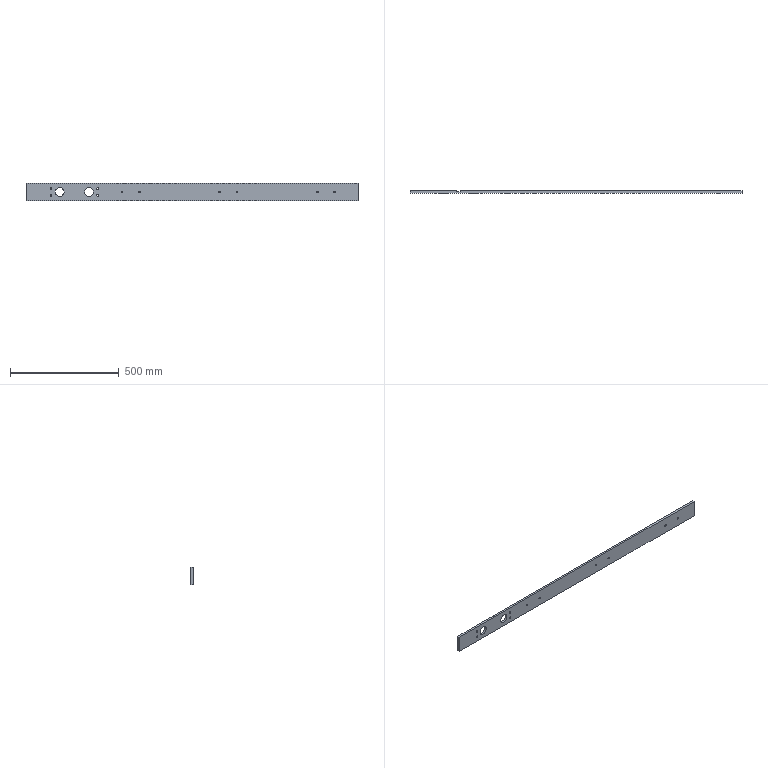Part | SolidWorks | features BaseBody 1 | 1 solid | 34 faces | box 1530 x 10 x 80 mm | volume 1186165 mm3 | cylinder 24 | plane 10 | commonest cylinder face diameters 8.5 x20 40.497 x4
STEP:
#1=CARTESIAN_POINT('',(-315.75,-7.,0.));
#2=VERTEX_POINT('',#1);
#3=CARTESIAN_POINT('',(-324.25,-7.,0.));
#4=VERTEX_POINT('',#3);
#5=CARTESIAN_POINT('',(-320.,-7.,0.));
#6=DIRECTION('',(0.,1.,0.));
#7=DIRECTION('',(0.,0.,1.));
#8=AXIS2_PLACEMENT_3D('',#5,#6,#7);
#9=CIRCLE('',#8,4.25);
#10=EDGE_CURVE('',#2,#4,#9,.T.);
#11=ORIENTED_EDGE('',*,*,#10,.F.);
#12=CARTESIAN_POINT('',(-315.75,3.,0.));
#13=VERTEX_POINT('',#12);
#14=CARTESIAN_POINT('',(-315.75,3.,0.));
#15=DIRECTION('',(0.,1.,0.));
#16=VECTOR('',#15,1000.);
#17=LINE('',#14,#16);
#18=EDGE_CURVE('',#2,#13,#17,.T.);
#19=ORIENTED_EDGE('',*,*,#18,.T.);
#20=CARTESIAN_POINT('',(-324.25,3.,0.));
#21=VERTEX_POINT('',#20);
#22=CARTESIAN_POINT('',(-320.,3.,0.));
#23=DIRECTION('',(0.,1.,0.));
#24=DIRECTION('',(-1.,0.,0.));
#25=AXIS2_PLACEMENT_3D('',#22,#23,#24);
#26=CIRCLE('',#25,4.25);
#27=EDGE_CURVE('',#13,#21,#26,.T.);
#28=ORIENTED_EDGE('',*,*,#27,.T.);
#29=CARTESIAN_POINT('',(-324.25,3.,0.));
#30=DIRECTION('',(0.,1.,0.));
#31=VECTOR('',#30,1000.);
#32=LINE('',#29,#31);
#33=EDGE_CURVE('',#4,#21,#32,.T.);
#34=ORIENTED_EDGE('',*,*,#33,.F.);
#35=EDGE_LOOP('',(#11,#19,#28,#34));
#36=FACE_OUTER_BOUND('',#35,.T.);
#37=CARTESIAN_POINT('',(-320.,3.,0.));
#38=DIRECTION('',(0.,1.,0.));
#39=DIRECTION('',(-1.,0.,0.));
#40=AXIS2_PLACEMENT_3D('',#37,#38,#39);
#41=CYLINDRICAL_SURFACE('',#40,4.25);
#42=ADVANCED_FACE('',(#36),#41,.F.);
#43=CARTESIAN_POINT('',(-235.75,-7.,0.));
#44=VERTEX_POINT('',#43);
#45=CARTESIAN_POINT('',(-244.25,-7.,0.));
#46=VERTEX_POINT('',#45);
#47=CARTESIAN_POINT('',(-240.,-7.,0.));
#48=DIRECTION('',(0.,1.,0.));
#49=DIRECTION('',(0.,0.,1.));
#50=AXIS2_PLACEMENT_3D('',#47,#48,#49);
#51=CIRCLE('',#50,4.25);
#52=EDGE_CURVE('',#44,#46,#51,.T.);
#53=ORIENTED_EDGE('',*,*,#52,.F.);
#54=CARTESIAN_POINT('',(-235.75,3.,0.));
#55=VERTEX_POINT('',#54);
#56=CARTESIAN_POINT('',(-235.75,3.,0.));
#57=DIRECTION('',(0.,1.,0.));
#58=VECTOR('',#57,1000.);
#59=LINE('',#56,#58);
#60=EDGE_CURVE('',#44,#55,#59,.T.);
#61=ORIENTED_EDGE('',*,*,#60,.T.);
#62=CARTESIAN_POINT('',(-244.25,3.,0.));
#63=VERTEX_POINT('',#62);
#64=CARTESIAN_POINT('',(-240.,3.,0.));
#65=DIRECTION('',(0.,1.,0.));
#66=DIRECTION('',(-1.,0.,0.));
#67=AXIS2_PLACEMENT_3D('',#64,#65,#66);
#68=CIRCLE('',#67,4.25);
#69=EDGE_CURVE('',#55,#63,#68,.T.);
#70=ORIENTED_EDGE('',*,*,#69,.T.);
#71=CARTESIAN_POINT('',(-244.25,3.,0.));
#72=DIRECTION('',(0.,1.,0.));
#73=VECTOR('',#72,1000.);
#74=LINE('',#71,#73);
#75=EDGE_CURVE('',#46,#63,#74,.T.);
#76=ORIENTED_EDGE('',*,*,#75,.F.);
#77=EDGE_LOOP('',(#53,#61,#70,#76));
#78=FACE_OUTER_BOUND('',#77,.T.);
#79=CARTESIAN_POINT('',(-240.,3.,0.));
#80=DIRECTION('',(0.,1.,0.));
#81=DIRECTION('',(-1.,0.,0.));
#82=AXIS2_PLACEMENT_3D('',#79,#80,#81);
#83=CYLINDRICAL_SURFACE('',#82,4.25);
#84=ADVANCED_FACE('',(#78),#83,.F.);
#85=CARTESIAN_POINT('',(134.25,-7.,0.));
#86=VERTEX_POINT('',#85);
#87=CARTESIAN_POINT('',(125.75,-7.,0.));
#88=VERTEX_POINT('',#87);
#89=CARTESIAN_POINT('',(130.,-7.,0.));
#90=DIRECTION('',(0.,1.,0.));
#91=DIRECTION('',(0.,0.,1.));
#92=AXIS2_PLACEMENT_3D('',#89,#90,#91);
#93=CIRCLE('',#92,4.25);
#94=EDGE_CURVE('',#86,#88,#93,.T.);
#95=ORIENTED_EDGE('',*,*,#94,.F.);
#96=CARTESIAN_POINT('',(134.25,3.,0.));
#97=VERTEX_POINT('',#96);
#98=CARTESIAN_POINT('',(134.25,3.,0.));
#99=DIRECTION('',(0.,1.,0.));
#100=VECTOR('',#99,1000.);
#101=LINE('',#98,#100);
#102=EDGE_CURVE('',#86,#97,#101,.T.);
#103=ORIENTED_EDGE('',*,*,#102,.T.);
#104=CARTESIAN_POINT('',(125.75,3.,0.));
#105=VERTEX_POINT('',#104);
#106=CARTESIAN_POINT('',(130.,3.,0.));
#107=DIRECTION('',(0.,1.,0.));
#108=DIRECTION('',(-1.,0.,0.));
#109=AXIS2_PLACEMENT_3D('',#106,#107,#108);
#110=CIRCLE('',#109,4.25);
#111=EDGE_CURVE('',#97,#105,#110,.T.);
#112=ORIENTED_EDGE('',*,*,#111,.T.);
#113=CARTESIAN_POINT('',(125.75,3.,0.));
#114=DIRECTION('',(0.,1.,0.));
#115=VECTOR('',#114,1000.);
#116=LINE('',#113,#115);
#117=EDGE_CURVE('',#88,#105,#116,.T.);
#118=ORIENTED_EDGE('',*,*,#117,.F.);
#119=EDGE_LOOP('',(#95,#103,#112,#118));
#120=FACE_OUTER_BOUND('',#119,.T.);
#121=CARTESIAN_POINT('',(130.,3.,0.));
#122=DIRECTION('',(0.,1.,0.));
#123=DIRECTION('',(-1.,0.,0.));
#124=AXIS2_PLACEMENT_3D('',#121,#122,#123);
#125=CYLINDRICAL_SURFACE('',#124,4.25);
#126=ADVANCED_FACE('',(#120),#125,.F.);
#127=CARTESIAN_POINT('',(214.25,-7.,0.));
#128=VERTEX_POINT('',#127);
#129=CARTESIAN_POINT('',(205.75,-7.,0.));
#130=VERTEX_POINT('',#129);
#131=CARTESIAN_POINT('',(210.,-7.,0.));
#132=DIRECTION('',(0.,1.,0.));
#133=DIRECTION('',(0.,0.,1.));
#134=AXIS2_PLACEMENT_3D('',#131,#132,#133);
#135=CIRCLE('',#134,4.25);
#136=EDGE_CURVE('',#128,#130,#135,.T.);
#137=ORIENTED_EDGE('',*,*,#136,.F.);
#138=CARTESIAN_POINT('',(214.25,3.,0.));
#139=VERTEX_POINT('',#138);
#140=CARTESIAN_POINT('',(214.25,3.,0.));
#141=DIRECTION('',(0.,1.,0.));
#142=VECTOR('',#141,1000.);
#143=LINE('',#140,#142);
#144=EDGE_CURVE('',#128,#139,#143,.T.);
#145=ORIENTED_EDGE('',*,*,#144,.T.);
#146=CARTESIAN_POINT('',(205.75,3.,0.));
#147=VERTEX_POINT('',#146);
#148=CARTESIAN_POINT('',(210.,3.,0.));
#149=DIRECTION('',(0.,1.,0.));
#150=DIRECTION('',(-1.,0.,0.));
#151=AXIS2_PLACEMENT_3D('',#148,#149,#150);
#152=CIRCLE('',#151,4.25);
#153=EDGE_CURVE('',#139,#147,#152,.T.);
#154=ORIENTED_EDGE('',*,*,#153,.T.);
#155=CARTESIAN_POINT('',(205.75,3.,0.));
#156=DIRECTION('',(0.,1.,0.));
#157=VECTOR('',#156,1000.);
#158=LINE('',#155,#157);
#159=EDGE_CURVE('',#130,#147,#158,.T.);
#160=ORIENTED_EDGE('',*,*,#159,.F.);
#161=EDGE_LOOP('',(#137,#145,#154,#160));
#162=FACE_OUTER_BOUND('',#161,.T.);
#163=CARTESIAN_POINT('',(210.,3.,0.));
#164=DIRECTION('',(0.,1.,0.));
#165=DIRECTION('',(-1.,0.,0.));
#166=AXIS2_PLACEMENT_3D('',#163,#164,#165);
#167=CYLINDRICAL_SURFACE('',#166,4.25);
#168=ADVANCED_FACE('',(#162),#167,.F.);
#169=CARTESIAN_POINT('',(584.25,-7.,0.));
#170=VERTEX_POINT('',#169);
#171=CARTESIAN_POINT('',(575.75,-7.,0.));
#172=VERTEX_POINT('',#171);
#173=CARTESIAN_POINT('',(580.,-7.,0.));
#174=DIRECTION('',(0.,1.,0.));
#175=DIRECTION('',(0.,0.,1.));
#176=AXIS2_PLACEMENT_3D('',#173,#174,#175);
#177=CIRCLE('',#176,4.25);
#178=EDGE_CURVE('',#170,#172,#177,.T.);
#179=ORIENTED_EDGE('',*,*,#178,.F.);
#180=CARTESIAN_POINT('',(584.25,3.,0.));
#181=VERTEX_POINT('',#180);
#182=CARTESIAN_POINT('',(584.25,3.,0.));
#183=DIRECTION('',(0.,1.,0.));
#184=VECTOR('',#183,1000.);
#185=LINE('',#182,#184);
#186=EDGE_CURVE('',#170,#181,#185,.T.);
#187=ORIENTED_EDGE('',*,*,#186,.T.);
#188=CARTESIAN_POINT('',(575.75,3.,0.));
#189=VERTEX_POINT('',#188);
#190=CARTESIAN_POINT('',(580.,3.,0.));
#191=DIRECTION('',(0.,1.,0.));
#192=DIRECTION('',(-1.,0.,0.));
#193=AXIS2_PLACEMENT_3D('',#190,#191,#192);
#194=CIRCLE('',#193,4.25);
#195=EDGE_CURVE('',#181,#189,#194,.T.);
#196=ORIENTED_EDGE('',*,*,#195,.T.);
#197=CARTESIAN_POINT('',(575.75,3.,0.));
#198=DIRECTION('',(0.,1.,0.));
#199=VECTOR('',#198,1000.);
#200=LINE('',#197,#199);
#201=EDGE_CURVE('',#172,#189,#200,.T.);
#202=ORIENTED_EDGE('',*,*,#201,.F.);
#203=EDGE_LOOP('',(#179,#187,#196,#202));
#204=FACE_OUTER_BOUND('',#203,.T.);
#205=CARTESIAN_POINT('',(580.,3.,0.));
#206=DIRECTION('',(0.,1.,0.));
#207=DIRECTION('',(-1.,0.,0.));
#208=AXIS2_PLACEMENT_3D('',#205,#206,#207);
#209=CYLINDRICAL_SURFACE('',#208,4.25);
#210=ADVANCED_FACE('',(#204),#209,.F.);
#211=CARTESIAN_POINT('',(664.25,-7.,0.));
#212=VERTEX_POINT('',#211);
#213=CARTESIAN_POINT('',(655.75,-7.,0.));
#214=VERTEX_POINT('',#213);
#215=CARTESIAN_POINT('',(660.,-7.,0.));
#216=DIRECTION('',(0.,1.,0.));
#217=DIRECTION('',(0.,0.,1.));
#218=AXIS2_PLACEMENT_3D('',#215,#216,#217);
#219=CIRCLE('',#218,4.25);
#220=EDGE_CURVE('',#212,#214,#219,.T.);
#221=ORIENTED_EDGE('',*,*,#220,.F.);
#222=CARTESIAN_POINT('',(664.25,3.,0.));
#223=VERTEX_POINT('',#222);
#224=CARTESIAN_POINT('',(664.25,3.,0.));
#225=DIRECTION('',(0.,1.,0.));
#226=VECTOR('',#225,1000.);
#227=LINE('',#224,#226);
#228=EDGE_CURVE('',#212,#223,#227,.T.);
#229=ORIENTED_EDGE('',*,*,#228,.T.);
#230=CARTESIAN_POINT('',(655.75,3.,0.));
#231=VERTEX_POINT('',#230);
#232=CARTESIAN_POINT('',(660.,3.,0.));
#233=DIRECTION('',(0.,1.,0.));
#234=DIRECTION('',(-1.,0.,0.));
#235=AXIS2_PLACEMENT_3D('',#232,#233,#234);
#236=CIRCLE('',#235,4.25);
#237=EDGE_CURVE('',#223,#231,#236,.T.);
#238=ORIENTED_EDGE('',*,*,#237,.T.);
#239=CARTESIAN_POINT('',(655.75,3.,0.));
#240=DIRECTION('',(0.,1.,0.));
#241=VECTOR('',#240,1000.);
#242=LINE('',#239,#241);
#243=EDGE_CURVE('',#214,#231,#242,.T.);
#244=ORIENTED_EDGE('',*,*,#243,.F.);
#245=EDGE_LOOP('',(#221,#229,#238,#244));
#246=FACE_OUTER_BOUND('',#245,.T.);
#247=CARTESIAN_POINT('',(660.,3.,0.));
#248=DIRECTION('',(0.,1.,0.));
#249=DIRECTION('',(-1.,0.,0.));
#250=AXIS2_PLACEMENT_3D('',#247,#248,#249);
#251=CYLINDRICAL_SURFACE('',#250,4.25);
#252=ADVANCED_FACE('',(#246),#251,.F.);
#253=CARTESIAN_POINT('',(-587.252,-7.,0.));
#254=VERTEX_POINT('',#253);
#255=CARTESIAN_POINT('',(-627.748,-7.,0.));
#256=VERTEX_POINT('',#255);
#257=CARTESIAN_POINT('',(-607.5,-7.,0.));
#258=DIRECTION('',(0.,1.,0.));
#259=DIRECTION('',(0.,0.,1.));
#260=AXIS2_PLACEMENT_3D('',#257,#258,#259);
#261=CIRCLE('',#260,20.248);
#262=EDGE_CURVE('',#254,#256,#261,.T.);
#263=ORIENTED_EDGE('',*,*,#262,.F.);
#264=CARTESIAN_POINT('',(-587.252,3.,0.));
#265=VERTEX_POINT('',#264);
#266=CARTESIAN_POINT('',(-587.252,-17.,0.));
#267=DIRECTION('',(0.,1.,0.));
#268=VECTOR('',#267,1000.);
#269=LINE('',#266,#268);
#270=EDGE_CURVE('',#254,#265,#269,.T.);
#271=ORIENTED_EDGE('',*,*,#270,.T.);
#272=CARTESIAN_POINT('',(-627.748,3.,0.));
#273=VERTEX_POINT('',#272);
#274=CARTESIAN_POINT('',(-607.5,3.,0.));
#275=DIRECTION('',(0.,1.,0.));
#276=DIRECTION('',(1.,0.,0.));
#277=AXIS2_PLACEMENT_3D('',#274,#275,#276);
#278=CIRCLE('',#277,20.248);
#279=EDGE_CURVE('',#265,#273,#278,.T.);
#280=ORIENTED_EDGE('',*,*,#279,.T.);
#281=CARTESIAN_POINT('',(-627.748,-17.,0.));
#282=DIRECTION('',(0.,1.,0.));
#283=VECTOR('',#282,1000.);
#284=LINE('',#281,#283);
#285=EDGE_CURVE('',#256,#273,#284,.T.);
#286=ORIENTED_EDGE('',*,*,#285,.F.);
#287=EDGE_LOOP('',(#263,#271,#280,#286));
#288=FACE_OUTER_BOUND('',#287,.T.);
#289=CARTESIAN_POINT('',(-607.5,-17.,0.));
#290=DIRECTION('',(0.,1.,0.));
#291=DIRECTION('',(-1.,0.,0.));
#292=AXIS2_PLACEMENT_3D('',#289,#290,#291);
#293=CYLINDRICAL_SURFACE('',#292,20.248);
#294=ADVANCED_FACE('',(#288),#293,.F.);
#295=CARTESIAN_POINT('',(-452.252,-7.,0.));
#296=VERTEX_POINT('',#295);
#297=CARTESIAN_POINT('',(-492.748,-7.,0.));
#298=VERTEX_POINT('',#297);
#299=CARTESIAN_POINT('',(-472.5,-7.,0.));
#300=DIRECTION('',(0.,1.,0.));
#301=DIRECTION('',(0.,0.,1.));
#302=AXIS2_PLACEMENT_3D('',#299,#300,#301);
#303=CIRCLE('',#302,20.248);
#304=EDGE_CURVE('',#296,#298,#303,.T.);
#305=ORIENTED_EDGE('',*,*,#304,.F.);
#306=CARTESIAN_POINT('',(-452.252,3.,0.));
#307=VERTEX_POINT('',#306);
#308=CARTESIAN_POINT('',(-452.252,-17.,0.));
#309=DIRECTION('',(0.,1.,0.));
#310=VECTOR('',#309,1000.);
#311=LINE('',#308,#310);
#312=EDGE_CURVE('',#296,#307,#311,.T.);
#313=ORIENTED_EDGE('',*,*,#312,.T.);
#314=CARTESIAN_POINT('',(-492.748,3.,0.));
#315=VERTEX_POINT('',#314);
#316=CARTESIAN_POINT('',(-472.5,3.,0.));
#317=DIRECTION('',(0.,1.,0.));
#318=DIRECTION('',(1.,0.,0.));
#319=AXIS2_PLACEMENT_3D('',#316,#317,#318);
#320=CIRCLE('',#319,20.248);
#321=EDGE_CURVE('',#307,#315,#320,.T.);
#322=ORIENTED_EDGE('',*,*,#321,.T.);
#323=CARTESIAN_POINT('',(-492.748,-17.,0.));
#324=DIRECTION('',(0.,1.,0.));
#325=VECTOR('',#324,1000.);
#326=LINE('',#323,#325);
#327=EDGE_CURVE('',#298,#315,#326,.T.);
#328=ORIENTED_EDGE('',*,*,#327,.F.);
#329=EDGE_LOOP('',(#305,#313,#322,#328));
#330=FACE_OUTER_BOUND('',#329,.T.);
#331=CARTESIAN_POINT('',(-472.5,-17.,0.));
#332=DIRECTION('',(0.,1.,0.));
#333=DIRECTION('',(-1.,0.,0.));
#334=AXIS2_PLACEMENT_3D('',#331,#332,#333);
#335=CYLINDRICAL_SURFACE('',#334,20.248);
#336=ADVANCED_FACE('',(#330),#335,.F.);
#337=CARTESIAN_POINT('',(-428.25,-7.,15.));
#338=VERTEX_POINT('',#337);
#339=CARTESIAN_POINT('',(-436.75,-7.,15.));
#340=VERTEX_POINT('',#339);
#341=CARTESIAN_POINT('',(-432.5,-7.,15.));
#342=DIRECTION('',(0.,1.,0.));
#343=DIRECTION('',(0.,0.,1.));
#344=AXIS2_PLACEMENT_3D('',#341,#342,#343);
#345=CIRCLE('',#344,4.25);
#346=EDGE_CURVE('',#338,#340,#345,.T.);
#347=ORIENTED_EDGE('',*,*,#346,.F.);
#348=CARTESIAN_POINT('',(-428.25,3.,15.));
#349=VERTEX_POINT('',#348);
#350=CARTESIAN_POINT('',(-428.25,3.,15.));
#351=DIRECTION('',(0.,1.,0.));
#352=VECTOR('',#351,1000.);
#353=LINE('',#350,#352);
#354=EDGE_CURVE('',#338,#349,#353,.T.);
#355=ORIENTED_EDGE('',*,*,#354,.T.);
#356=CARTESIAN_POINT('',(-436.75,3.,15.));
#357=VERTEX_POINT('',#356);
#358=CARTESIAN_POINT('',(-432.5,3.,15.));
#359=DIRECTION('',(0.,1.,0.));
#360=DIRECTION('',(-1.,0.,0.));
#361=AXIS2_PLACEMENT_3D('',#358,#359,#360);
#362=CIRCLE('',#361,4.25);
#363=EDGE_CURVE('',#349,#357,#362,.T.);
#364=ORIENTED_EDGE('',*,*,#363,.T.);
#365=CARTESIAN_POINT('',(-436.75,3.,15.));
#366=DIRECTION('',(0.,1.,0.));
#367=VECTOR('',#366,1000.);
#368=LINE('',#365,#367);
#369=EDGE_CURVE('',#340,#357,#368,.T.);
#370=ORIENTED_EDGE('',*,*,#369,.F.);
#371=EDGE_LOOP('',(#347,#355,#364,#370));
#372=FACE_OUTER_BOUND('',#371,.T.);
#373=CARTESIAN_POINT('',(-432.5,3.,15.));
#374=DIRECTION('',(0.,1.,0.));
#375=DIRECTION('',(-1.,0.,0.));
#376=AXIS2_PLACEMENT_3D('',#373,#374,#375);
#377=CYLINDRICAL_SURFACE('',#376,4.25);
#378=ADVANCED_FACE('',(#372),#377,.F.);
#379=CARTESIAN_POINT('',(-428.25,-7.,-15.));
#380=VERTEX_POINT('',#379);
#381=CARTESIAN_POINT('',(-436.75,-7.,-15.));
#382=VERTEX_POINT('',#381);
#383=CARTESIAN_POINT('',(-432.5,-7.,-15.));
#384=DIRECTION('',(0.,1.,0.));
#385=DIRECTION('',(0.,0.,1.));
#386=AXIS2_PLACEMENT_3D('',#383,#384,#385);
#387=CIRCLE('',#386,4.25);
#388=EDGE_CURVE('',#380,#382,#387,.T.);
#389=ORIENTED_EDGE('',*,*,#388,.F.);
#390=CARTESIAN_POINT('',(-428.25,3.,-15.));
#391=VERTEX_POINT('',#390);
#392=CARTESIAN_POINT('',(-428.25,3.,-15.));
#393=DIRECTION('',(0.,1.,0.));
#394=VECTOR('',#393,1000.);
#395=LINE('',#392,#394);
#396=EDGE_CURVE('',#380,#391,#395,.T.);
#397=ORIENTED_EDGE('',*,*,#396,.T.);
#398=CARTESIAN_POINT('',(-436.75,3.,-15.));
#399=VERTEX_POINT('',#398);
#400=CARTESIAN_POINT('',(-432.5,3.,-15.));
#401=DIRECTION('',(0.,1.,0.));
#402=DIRECTION('',(-1.,0.,0.));
#403=AXIS2_PLACEMENT_3D('',#400,#401,#402);
#404=CIRCLE('',#403,4.25);
#405=EDGE_CURVE('',#391,#399,#404,.T.);
#406=ORIENTED_EDGE('',*,*,#405,.T.);
#407=CARTESIAN_POINT('',(-436.75,3.,-15.));
#408=DIRECTION('',(0.,1.,0.));
#409=VECTOR('',#408,1000.);
#410=LINE('',#407,#409);
#411=EDGE_CURVE('',#382,#399,#410,.T.);
#412=ORIENTED_EDGE('',*,*,#411,.F.);
#413=EDGE_LOOP('',(#389,#397,#406,#412));
#414=FACE_OUTER_BOUND('',#413,.T.);
#415=CARTESIAN_POINT('',(-432.5,3.,-15.));
#416=DIRECTION('',(0.,1.,0.));
#417=DIRECTION('',(-1.,0.,0.));
#418=AXIS2_PLACEMENT_3D('',#415,#416,#417);
#419=CYLINDRICAL_SURFACE('',#418,4.25);
#420=ADVANCED_FACE('',(#414),#419,.F.);
#421=CARTESIAN_POINT('',(-643.25,-7.,-15.));
#422=VERTEX_POINT('',#421);
#423=CARTESIAN_POINT('',(-651.75,-7.,-15.));
#424=VERTEX_POINT('',#423);
#425=CARTESIAN_POINT('',(-647.5,-7.,-15.));
#426=DIRECTION('',(0.,1.,0.));
#427=DIRECTION('',(0.,0.,1.));
#428=AXIS2_PLACEMENT_3D('',#425,#426,#427);
#429=CIRCLE('',#428,4.25);
#430=EDGE_CURVE('',#422,#424,#429,.T.);
#431=ORIENTED_EDGE('',*,*,#430,.F.);
#432=CARTESIAN_POINT('',(-643.25,3.,-15.));
#433=VERTEX_POINT('',#432);
#434=CARTESIAN_POINT('',(-643.25,3.,-15.));
#435=DIRECTION('',(0.,1.,0.));
#436=VECTOR('',#435,1000.);
#437=LINE('',#434,#436);
#438=EDGE_CURVE('',#422,#433,#437,.T.);
#439=ORIENTED_EDGE('',*,*,#438,.T.);
#440=CARTESIAN_POINT('',(-651.75,3.,-15.));
#441=VERTEX_POINT('',#440);
#442=CARTESIAN_POINT('',(-647.5,3.,-15.));
#443=DIRECTION('',(0.,1.,0.));
#444=DIRECTION('',(-1.,0.,0.));
#445=AXIS2_PLACEMENT_3D('',#442,#443,#444);
#446=CIRCLE('',#445,4.25);
#447=EDGE_CURVE('',#433,#441,#446,.T.);
#448=ORIENTED_EDGE('',*,*,#447,.T.);
#449=CARTESIAN_POINT('',(-651.75,3.,-15.));
#450=DIRECTION('',(0.,1.,0.));
#451=VECTOR('',#450,1000.);
#452=LINE('',#449,#451);
#453=EDGE_CURVE('',#424,#441,#452,.T.);
#454=ORIENTED_EDGE('',*,*,#453,.F.);
#455=EDGE_LOOP('',(#431,#439,#448,#454));
#456=FACE_OUTER_BOUND('',#455,.T.);
#457=CARTESIAN_POINT('',(-647.5,3.,-15.));
#458=DIRECTION('',(0.,1.,0.));
#459=DIRECTION('',(-1.,0.,0.));
#460=AXIS2_PLACEMENT_3D('',#457,#458,#459);
#461=CYLINDRICAL_SURFACE('',#460,4.25);
#462=ADVANCED_FACE('',(#456),#461,.F.);
#463=CARTESIAN_POINT('',(-643.25,-7.,15.));
#464=VERTEX_POINT('',#463);
#465=CARTESIAN_POINT('',(-651.75,-7.,15.));
#466=VERTEX_POINT('',#465);
#467=CARTESIAN_POINT('',(-647.5,-7.,15.));
#468=DIRECTION('',(0.,1.,0.));
#469=DIRECTION('',(0.,0.,1.));
#470=AXIS2_PLACEMENT_3D('',#467,#468,#469);
#471=CIRCLE('',#470,4.25);
#472=EDGE_CURVE('',#464,#466,#471,.T.);
#473=ORIENTED_EDGE('',*,*,#472,.F.);
#474=CARTESIAN_POINT('',(-643.25,3.,15.));
#475=VERTEX_POINT('',#474);
#476=CARTESIAN_POINT('',(-643.25,3.,15.));
#477=DIRECTION('',(0.,1.,0.));
#478=VECTOR('',#477,1000.);
#479=LINE('',#476,#478);
#480=EDGE_CURVE('',#464,#475,#479,.T.);
#481=ORIENTED_EDGE('',*,*,#480,.T.);
#482=CARTESIAN_POINT('',(-651.75,3.,15.));
#483=VERTEX_POINT('',#482);
#484=CARTESIAN_POINT('',(-647.5,3.,15.));
#485=DIRECTION('',(0.,1.,0.));
#486=DIRECTION('',(-1.,0.,0.));
#487=AXIS2_PLACEMENT_3D('',#484,#485,#486);
#488=CIRCLE('',#487,4.25);
#489=EDGE_CURVE('',#475,#483,#488,.T.);
#490=ORIENTED_EDGE('',*,*,#489,.T.);
#491=CARTESIAN_POINT('',(-651.75,3.,15.));
#492=DIRECTION('',(0.,1.,0.));
#493=VECTOR('',#492,1000.);
#494=LINE('',#491,#493);
#495=EDGE_CURVE('',#466,#483,#494,.T.);
#496=ORIENTED_EDGE('',*,*,#495,.F.);
#497=EDGE_LOOP('',(#473,#481,#490,#496));
#498=FACE_OUTER_BOUND('',#497,.T.);
#499=CARTESIAN_POINT('',(-647.5,3.,15.));
#500=DIRECTION('',(0.,1.,0.));
#501=DIRECTION('',(-1.,0.,0.));
#502=AXIS2_PLACEMENT_3D('',#499,#500,#501);
#503=CYLINDRICAL_SURFACE('',#502,4.25);
#504=ADVANCED_FACE('',(#498),#503,.F.);
#505=CARTESIAN_POINT('',(-548.,3.,-40.));
#506=VERTEX_POINT('',#505);
#507=CARTESIAN_POINT('',(-548.,3.,40.));
#508=VERTEX_POINT('',#507);
#509=CARTESIAN_POINT('',(-548.,3.,40.));
#510=DIRECTION('',(0.,0.,1.));
#511=VECTOR('',#510,1000.);
#512=LINE('',#509,#511);
#513=EDGE_CURVE('',#506,#508,#512,.T.);
#514=ORIENTED_EDGE('',*,*,#513,.F.);
#515=CARTESIAN_POINT('',(-762.5,3.,-40.));
#516=VERTEX_POINT('',#515);
#517=CARTESIAN_POINT('',(-767.5,3.,-40.));
#518=DIRECTION('',(-1.,0.,0.));
#519=VECTOR('',#518,1000.);
#520=LINE('',#517,#519);
#521=EDGE_CURVE('',#506,#516,#520,.T.);
#522=ORIENTED_EDGE('',*,*,#521,.T.);
#523=CARTESIAN_POINT('',(-762.5,3.,40.));
#524=VERTEX_POINT('',#523);
#525=CARTESIAN_POINT('',(-762.5,3.,-1390.));
#526=DIRECTION('',(0.,0.,-1.));
#527=VECTOR('',#526,1000.);
#528=LINE('',#525,#527);
#529=EDGE_CURVE('',#524,#516,#528,.T.);
#530=ORIENTED_EDGE('',*,*,#529,.F.);
#531=CARTESIAN_POINT('',(767.5,3.,40.));
#532=DIRECTION('',(1.,0.,0.));
#533=VECTOR('',#532,1000.);
#534=LINE('',#531,#533);
#535=EDGE_CURVE('',#524,#508,#534,.T.);
#536=ORIENTED_EDGE('',*,*,#535,.T.);
#537=EDGE_LOOP('',(#514,#522,#530,#536));
#538=FACE_OUTER_BOUND('',#537,.T.);
#539=CARTESIAN_POINT('',(-647.5,3.,15.));
#540=DIRECTION('',(0.,1.,0.));
#541=DIRECTION('',(-1.,0.,0.));
#542=AXIS2_PLACEMENT_3D('',#539,#540,#541);
#543=CIRCLE('',#542,4.25);
#544=EDGE_CURVE('',#483,#475,#543,.T.);
#545=ORIENTED_EDGE('',*,*,#544,.F.);
#546=ORIENTED_EDGE('',*,*,#489,.F.);
#547=EDGE_LOOP('',(#545,#546));
#548=FACE_BOUND('',#547,.T.);
#549=CARTESIAN_POINT('',(-647.5,3.,-15.));
#550=DIRECTION('',(0.,1.,0.));
#551=DIRECTION('',(-1.,0.,0.));
#552=AXIS2_PLACEMENT_3D('',#549,#550,#551);
#553=CIRCLE('',#552,4.25);
#554=EDGE_CURVE('',#441,#433,#553,.T.);
#555=ORIENTED_EDGE('',*,*,#554,.F.);
#556=ORIENTED_EDGE('',*,*,#447,.F.);
#557=EDGE_LOOP('',(#555,#556));
#558=FACE_BOUND('',#557,.T.);
#559=CARTESIAN_POINT('',(-607.5,3.,0.));
#560=DIRECTION('',(0.,1.,0.));
#561=DIRECTION('',(1.,0.,0.));
#562=AXIS2_PLACEMENT_3D('',#559,#560,#561);
#563=CIRCLE('',#562,20.248);
#564=EDGE_CURVE('',#273,#265,#563,.T.);
#565=ORIENTED_EDGE('',*,*,#564,.F.);
#566=ORIENTED_EDGE('',*,*,#279,.F.);
#567=EDGE_LOOP('',(#565,#566));
#568=FACE_BOUND('',#567,.T.);
#569=CARTESIAN_POINT('',(0.,3.,-675.));
#570=DIRECTION('',(0.,1.,0.));
#571=DIRECTION('',(-1.,0.,0.));
#572=AXIS2_PLACEMENT_3D('',#569,#570,#571);
#573=PLANE('',#572);
#574=ADVANCED_FACE('',(#538,#548,#558,#568),#573,.T.);
#575=ORIENTED_EDGE('',*,*,#521,.F.);
#576=CARTESIAN_POINT('',(-548.,-2.,-40.));
#577=VERTEX_POINT('',#576);
#578=CARTESIAN_POINT('',(-548.,-2.,-40.));
#579=DIRECTION('',(0.,1.,0.));
#580=VECTOR('',#579,1000.);
#581=LINE('',#578,#580);
#582=EDGE_CURVE('',#577,#506,#581,.T.);
#583=ORIENTED_EDGE('',*,*,#582,.F.);
#584=CARTESIAN_POINT('',(-532.,-2.,-40.));
#585=VERTEX_POINT('',#584);
#586=CARTESIAN_POINT('',(-767.5,-2.,-40.));
#587=DIRECTION('',(1.,0.,0.));
#588=VECTOR('',#587,1000.);
#589=LINE('',#586,#588);
#590=EDGE_CURVE('',#577,#585,#589,.T.);
#591=ORIENTED_EDGE('',*,*,#590,.T.);
#592=CARTESIAN_POINT('',(-532.,3.,-40.));
#593=VERTEX_POINT('',#592);
#594=CARTESIAN_POINT('',(-532.,-2.,-40.));
#595=DIRECTION('',(0.,1.,0.));
#596=VECTOR('',#595,1000.);
#597=LINE('',#594,#596);
#598=EDGE_CURVE('',#585,#593,#597,.T.);
#599=ORIENTED_EDGE('',*,*,#598,.T.);
#600=CARTESIAN_POINT('',(767.5,3.,-40.));
#601=VERTEX_POINT('',#600);
#602=CARTESIAN_POINT('',(-767.5,3.,-40.));
#603=DIRECTION('',(-1.,0.,0.));
#604=VECTOR('',#603,1000.);
#605=LINE('',#602,#604);
#606=EDGE_CURVE('',#601,#593,#605,.T.);
#607=ORIENTED_EDGE('',*,*,#606,.F.);
#608=CARTESIAN_POINT('',(767.5,-7.,-40.));
#609=VERTEX_POINT('',#608);
#610=CARTESIAN_POINT('',(767.5,7.,-40.));
#611=DIRECTION('',(0.,-1.,0.));
#612=VECTOR('',#611,1000.);
#613=LINE('',#610,#612);
#614=EDGE_CURVE('',#601,#609,#613,.T.);
#615=ORIENTED_EDGE('',*,*,#614,.T.);
#616=CARTESIAN_POINT('',(-762.5,-7.,-40.));
#617=VERTEX_POINT('',#616);
#618=CARTESIAN_POINT('',(-767.5,-7.,-40.));
#619=DIRECTION('',(-1.,0.,0.));
#620=VECTOR('',#619,1000.);
#621=LINE('',#618,#620);
#622=EDGE_CURVE('',#609,#617,#621,.T.);
#623=ORIENTED_EDGE('',*,*,#622,.T.);
#624=CARTESIAN_POINT('',(-762.5,7.,-40.));
#625=DIRECTION('',(0.,-1.,0.));
#626=VECTOR('',#625,1000.);
#627=LINE('',#624,#626);
#628=EDGE_CURVE('',#516,#617,#627,.T.);
#629=ORIENTED_EDGE('',*,*,#628,.F.);
#630=EDGE_LOOP('',(#575,#583,#591,#599,#607,#615,#623,#629));
#631=FACE_OUTER_BOUND('',#630,.T.);
#632=CARTESIAN_POINT('',(-767.5,7.,-40.));
#633=DIRECTION('',(0.,0.,1.));
#634=DIRECTION('',(1.,0.,0.));
#635=AXIS2_PLACEMENT_3D('',#632,#633,#634);
#636=PLANE('',#635);
#637=ADVANCED_FACE('',(#631),#636,.F.);
#638=CARTESIAN_POINT('',(-532.,-2.,40.));
#639=VERTEX_POINT('',#638);
#640=CARTESIAN_POINT('',(-548.,-2.,40.));
#641=VERTEX_POINT('',#640);
#642=CARTESIAN_POINT('',(-767.5,-2.,40.));
#643=DIRECTION('',(-1.,0.,0.));
#644=VECTOR('',#643,1000.);
#645=LINE('',#642,#644);
#646=EDGE_CURVE('',#639,#641,#645,.T.);
#647=ORIENTED_EDGE('',*,*,#646,.T.);
#648=CARTESIAN_POINT('',(-548.,-2.,40.));
#649=DIRECTION('',(0.,1.,0.));
#650=VECTOR('',#649,1000.);
#651=LINE('',#648,#650);
#652=EDGE_CURVE('',#641,#508,#651,.T.);
#653=ORIENTED_EDGE('',*,*,#652,.T.);
#654=ORIENTED_EDGE('',*,*,#535,.F.);
#655=CARTESIAN_POINT('',(-762.5,-7.,40.));
#656=VERTEX_POINT('',#655);
#657=CARTESIAN_POINT('',(-762.5,3.,40.));
#658=DIRECTION('',(0.,1.,0.));
#659=VECTOR('',#658,1000.);
#660=LINE('',#657,#659);
#661=EDGE_CURVE('',#656,#524,#660,.T.);
#662=ORIENTED_EDGE('',*,*,#661,.F.);
#663=CARTESIAN_POINT('',(767.5,-7.,40.));
#664=VERTEX_POINT('',#663);
#665=CARTESIAN_POINT('',(-767.5,-7.,40.));
#666=DIRECTION('',(1.,0.,0.));
#667=VECTOR('',#666,1000.);
#668=LINE('',#665,#667);
#669=EDGE_CURVE('',#656,#664,#668,.T.);
#670=ORIENTED_EDGE('',*,*,#669,.T.);
#671=CARTESIAN_POINT('',(767.5,3.,40.));
#672=VERTEX_POINT('',#671);
#673=CARTESIAN_POINT('',(767.5,7.,40.));
#674=DIRECTION('',(0.,-1.,0.));
#675=VECTOR('',#674,1000.);
#676=LINE('',#673,#675);
#677=EDGE_CURVE('',#672,#664,#676,.T.);
#678=ORIENTED_EDGE('',*,*,#677,.F.);
#679=CARTESIAN_POINT('',(-532.,3.,40.));
#680=VERTEX_POINT('',#679);
#681=CARTESIAN_POINT('',(767.5,3.,40.));
#682=DIRECTION('',(1.,0.,0.));
#683=VECTOR('',#682,1000.);
#684=LINE('',#681,#683);
#685=EDGE_CURVE('',#680,#672,#684,.T.);
#686=ORIENTED_EDGE('',*,*,#685,.F.);
#687=CARTESIAN_POINT('',(-532.,-2.,40.));
#688=DIRECTION('',(0.,1.,0.));
#689=VECTOR('',#688,1000.);
#690=LINE('',#687,#689);
#691=EDGE_CURVE('',#639,#680,#690,.T.);
#692=ORIENTED_EDGE('',*,*,#691,.F.);
#693=EDGE_LOOP('',(#647,#653,#654,#662,#670,#678,#686,#692));
#694=FACE_OUTER_BOUND('',#693,.T.);
#695=CARTESIAN_POINT('',(-767.5,7.,40.));
#696=DIRECTION('',(0.,0.,-1.));
#697=DIRECTION('',(-1.,0.,0.));
#698=AXIS2_PLACEMENT_3D('',#695,#696,#697);
#699=PLANE('',#698);
#700=ADVANCED_FACE('',(#694),#699,.F.);
#701=CARTESIAN_POINT('',(-320.,-7.,0.));
#702=DIRECTION('',(0.,1.,0.));
#703=DIRECTION('',(0.,0.,1.));
#704=AXIS2_PLACEMENT_3D('',#701,#702,#703);
#705=CIRCLE('',#704,4.25);
#706=EDGE_CURVE('',#4,#2,#705,.T.);
#707=ORIENTED_EDGE('',*,*,#706,.T.);
#708=ORIENTED_EDGE('',*,*,#10,.T.);
#709=EDGE_LOOP('',(#707,#708));
#710=FACE_BOUND('',#709,.T.);
#711=CARTESIAN_POINT('',(-240.,-7.,0.));
#712=DIRECTION('',(0.,1.,0.));
#713=DIRECTION('',(0.,0.,1.));
#714=AXIS2_PLACEMENT_3D('',#711,#712,#713);
#715=CIRCLE('',#714,4.25);
#716=EDGE_CURVE('',#46,#44,#715,.T.);
#717=ORIENTED_EDGE('',*,*,#716,.T.);
#718=ORIENTED_EDGE('',*,*,#52,.T.);
#719=EDGE_LOOP('',(#717,#718));
#720=FACE_BOUND('',#719,.T.);
#721=CARTESIAN_POINT('',(130.,-7.,0.));
#722=DIRECTION('',(0.,1.,0.));
#723=DIRECTION('',(0.,0.,1.));
#724=AXIS2_PLACEMENT_3D('',#721,#722,#723);
#725=CIRCLE('',#724,4.25);
#726=EDGE_CURVE('',#88,#86,#725,.T.);
#727=ORIENTED_EDGE('',*,*,#726,.T.);
#728=ORIENTED_EDGE('',*,*,#94,.T.);
#729=EDGE_LOOP('',(#727,#728));
#730=FACE_BOUND('',#729,.T.);
#731=CARTESIAN_POINT('',(210.,-7.,0.));
#732=DIRECTION('',(0.,1.,0.));
#733=DIRECTION('',(0.,0.,1.));
#734=AXIS2_PLACEMENT_3D('',#731,#732,#733);
#735=CIRCLE('',#734,4.25);
#736=EDGE_CURVE('',#130,#128,#735,.T.);
#737=ORIENTED_EDGE('',*,*,#736,.T.);
#738=ORIENTED_EDGE('',*,*,#136,.T.);
#739=EDGE_LOOP('',(#737,#738));
#740=FACE_BOUND('',#739,.T.);
#741=CARTESIAN_POINT('',(580.,-7.,0.));
#742=DIRECTION('',(0.,1.,0.));
#743=DIRECTION('',(0.,0.,1.));
#744=AXIS2_PLACEMENT_3D('',#741,#742,#743);
#745=CIRCLE('',#744,4.25);
#746=EDGE_CURVE('',#172,#170,#745,.T.);
#747=ORIENTED_EDGE('',*,*,#746,.T.);
#748=ORIENTED_EDGE('',*,*,#178,.T.);
#749=EDGE_LOOP('',(#747,#748));
#750=FACE_BOUND('',#749,.T.);
#751=CARTESIAN_POINT('',(660.,-7.,0.));
#752=DIRECTION('',(0.,1.,0.));
#753=DIRECTION('',(0.,0.,1.));
#754=AXIS2_PLACEMENT_3D('',#751,#752,#753);
#755=CIRCLE('',#754,4.25);
#756=EDGE_CURVE('',#214,#212,#755,.T.);
#757=ORIENTED_EDGE('',*,*,#756,.T.);
#758=ORIENTED_EDGE('',*,*,#220,.T.);
#759=EDGE_LOOP('',(#757,#758));
#760=FACE_BOUND('',#759,.T.);
#761=CARTESIAN_POINT('',(-607.5,-7.,0.));
#762=DIRECTION('',(0.,1.,0.));
#763=DIRECTION('',(0.,0.,1.));
#764=AXIS2_PLACEMENT_3D('',#761,#762,#763);
#765=CIRCLE('',#764,20.248);
#766=EDGE_CURVE('',#256,#254,#765,.T.);
#767=ORIENTED_EDGE('',*,*,#766,.T.);
#768=ORIENTED_EDGE('',*,*,#262,.T.);
#769=EDGE_LOOP('',(#767,#768));
#770=FACE_BOUND('',#769,.T.);
#771=CARTESIAN_POINT('',(-472.5,-7.,0.));
#772=DIRECTION('',(0.,1.,0.));
#773=DIRECTION('',(0.,0.,1.));
#774=AXIS2_PLACEMENT_3D('',#771,#772,#773);
#775=CIRCLE('',#774,20.248);
#776=EDGE_CURVE('',#298,#296,#775,.T.);
#777=ORIENTED_EDGE('',*,*,#776,.T.);
#778=ORIENTED_EDGE('',*,*,#304,.T.);
#779=EDGE_LOOP('',(#777,#778));
#780=FACE_BOUND('',#779,.T.);
#781=CARTESIAN_POINT('',(-432.5,-7.,15.));
#782=DIRECTION('',(0.,1.,0.));
#783=DIRECTION('',(0.,0.,1.));
#784=AXIS2_PLACEMENT_3D('',#781,#782,#783);
#785=CIRCLE('',#784,4.25);
#786=EDGE_CURVE('',#340,#338,#785,.T.);
#787=ORIENTED_EDGE('',*,*,#786,.T.);
#788=ORIENTED_EDGE('',*,*,#346,.T.);
#789=EDGE_LOOP('',(#787,#788));
#790=FACE_BOUND('',#789,.T.);
#791=CARTESIAN_POINT('',(-432.5,-7.,-15.));
#792=DIRECTION('',(0.,1.,0.));
#793=DIRECTION('',(0.,0.,1.));
#794=AXIS2_PLACEMENT_3D('',#791,#792,#793);
#795=CIRCLE('',#794,4.25);
#796=EDGE_CURVE('',#382,#380,#795,.T.);
#797=ORIENTED_EDGE('',*,*,#796,.T.);
#798=ORIENTED_EDGE('',*,*,#388,.T.);
#799=EDGE_LOOP('',(#797,#798));
#800=FACE_BOUND('',#799,.T.);
#801=CARTESIAN_POINT('',(-647.5,-7.,-15.));
#802=DIRECTION('',(0.,1.,0.));
#803=DIRECTION('',(0.,0.,1.));
#804=AXIS2_PLACEMENT_3D('',#801,#802,#803);
#805=CIRCLE('',#804,4.25);
#806=EDGE_CURVE('',#424,#422,#805,.T.);
#807=ORIENTED_EDGE('',*,*,#806,.T.);
#808=ORIENTED_EDGE('',*,*,#430,.T.);
#809=EDGE_LOOP('',(#807,#808));
#810=FACE_BOUND('',#809,.T.);
#811=CARTESIAN_POINT('',(-647.5,-7.,15.));
#812=DIRECTION('',(0.,1.,0.));
#813=DIRECTION('',(0.,0.,1.));
#814=AXIS2_PLACEMENT_3D('',#811,#812,#813);
#815=CIRCLE('',#814,4.25);
#816=EDGE_CURVE('',#466,#464,#815,.T.);
#817=ORIENTED_EDGE('',*,*,#816,.T.);
#818=ORIENTED_EDGE('',*,*,#472,.T.);
#819=EDGE_LOOP('',(#817,#818));
#820=FACE_BOUND('',#819,.T.);
#821=CARTESIAN_POINT('',(-762.5,-7.,0.));
#822=DIRECTION('',(0.,0.,1.));
#823=VECTOR('',#822,1000.);
#824=LINE('',#821,#823);
#825=EDGE_CURVE('',#617,#656,#824,.T.);
#826=ORIENTED_EDGE('',*,*,#825,.F.);
#827=ORIENTED_EDGE('',*,*,#622,.F.);
#828=CARTESIAN_POINT('',(767.5,-7.,-40.));
#829=DIRECTION('',(0.,0.,-1.));
#830=VECTOR('',#829,1000.);
#831=LINE('',#828,#830);
#832=EDGE_CURVE('',#664,#609,#831,.T.);
#833=ORIENTED_EDGE('',*,*,#832,.F.);
#834=ORIENTED_EDGE('',*,*,#669,.F.);
#835=EDGE_LOOP('',(#826,#827,#833,#834));
#836=FACE_OUTER_BOUND('',#835,.T.);
#837=CARTESIAN_POINT('',(0.,-7.,0.));
#838=DIRECTION('',(0.,1.,0.));
#839=DIRECTION('',(0.,0.,1.));
#840=AXIS2_PLACEMENT_3D('',#837,#838,#839);
#841=PLANE('',#840);
#842=ADVANCED_FACE('',(#710,#720,#730,#740,#750,#760,#770,#780,#790,#800,#810,#820,#836),#841,.F.);
#843=CARTESIAN_POINT('',(-320.,3.,0.));
#844=DIRECTION('',(0.,1.,0.));
#845=DIRECTION('',(-1.,0.,0.));
#846=AXIS2_PLACEMENT_3D('',#843,#844,#845);
#847=CIRCLE('',#846,4.25);
#848=EDGE_CURVE('',#21,#13,#847,.T.);
#849=ORIENTED_EDGE('',*,*,#848,.F.);
#850=ORIENTED_EDGE('',*,*,#27,.F.);
#851=EDGE_LOOP('',(#849,#850));
#852=FACE_BOUND('',#851,.T.);
#853=CARTESIAN_POINT('',(-240.,3.,0.));
#854=DIRECTION('',(0.,1.,0.));
#855=DIRECTION('',(-1.,0.,0.));
#856=AXIS2_PLACEMENT_3D('',#853,#854,#855);
#857=CIRCLE('',#856,4.25);
#858=EDGE_CURVE('',#63,#55,#857,.T.);
#859=ORIENTED_EDGE('',*,*,#858,.F.);
#860=ORIENTED_EDGE('',*,*,#69,.F.);
#861=EDGE_LOOP('',(#859,#860));
#862=FACE_BOUND('',#861,.T.);
#863=CARTESIAN_POINT('',(130.,3.,0.));
#864=DIRECTION('',(0.,1.,0.));
#865=DIRECTION('',(-1.,0.,0.));
#866=AXIS2_PLACEMENT_3D('',#863,#864,#865);
#867=CIRCLE('',#866,4.25);
#868=EDGE_CURVE('',#105,#97,#867,.T.);
#869=ORIENTED_EDGE('',*,*,#868,.F.);
#870=ORIENTED_EDGE('',*,*,#111,.F.);
#871=EDGE_LOOP('',(#869,#870));
#872=FACE_BOUND('',#871,.T.);
#873=CARTESIAN_POINT('',(210.,3.,0.));
#874=DIRECTION('',(0.,1.,0.));
#875=DIRECTION('',(-1.,0.,0.));
#876=AXIS2_PLACEMENT_3D('',#873,#874,#875);
#877=CIRCLE('',#876,4.25);
#878=EDGE_CURVE('',#147,#139,#877,.T.);
#879=ORIENTED_EDGE('',*,*,#878,.F.);
#880=ORIENTED_EDGE('',*,*,#153,.F.);
#881=EDGE_LOOP('',(#879,#880));
#882=FACE_BOUND('',#881,.T.);
#883=CARTESIAN_POINT('',(580.,3.,0.));
#884=DIRECTION('',(0.,1.,0.));
#885=DIRECTION('',(-1.,0.,0.));
#886=AXIS2_PLACEMENT_3D('',#883,#884,#885);
#887=CIRCLE('',#886,4.25);
#888=EDGE_CURVE('',#189,#181,#887,.T.);
#889=ORIENTED_EDGE('',*,*,#888,.F.);
#890=ORIENTED_EDGE('',*,*,#195,.F.);
#891=EDGE_LOOP('',(#889,#890));
#892=FACE_BOUND('',#891,.T.);
#893=CARTESIAN_POINT('',(660.,3.,0.));
#894=DIRECTION('',(0.,1.,0.));
#895=DIRECTION('',(-1.,0.,0.));
#896=AXIS2_PLACEMENT_3D('',#893,#894,#895);
#897=CIRCLE('',#896,4.25);
#898=EDGE_CURVE('',#231,#223,#897,.T.);
#899=ORIENTED_EDGE('',*,*,#898,.F.);
#900=ORIENTED_EDGE('',*,*,#237,.F.);
#901=EDGE_LOOP('',(#899,#900));
#902=FACE_BOUND('',#901,.T.);
#903=CARTESIAN_POINT('',(-532.,3.,40.));
#904=DIRECTION('',(0.,0.,-1.));
#905=VECTOR('',#904,1000.);
#906=LINE('',#903,#905);
#907=EDGE_CURVE('',#680,#593,#906,.T.);
#908=ORIENTED_EDGE('',*,*,#907,.F.);
#909=ORIENTED_EDGE('',*,*,#685,.T.);
#910=CARTESIAN_POINT('',(767.5,3.,-1390.));
#911=DIRECTION('',(0.,0.,-1.));
#912=VECTOR('',#911,1000.);
#913=LINE('',#910,#912);
#914=EDGE_CURVE('',#672,#601,#913,.T.);
#915=ORIENTED_EDGE('',*,*,#914,.T.);
#916=ORIENTED_EDGE('',*,*,#606,.T.);
#917=EDGE_LOOP('',(#908,#909,#915,#916));
#918=FACE_OUTER_BOUND('',#917,.T.);
#919=CARTESIAN_POINT('',(-472.5,3.,0.));
#920=DIRECTION('',(0.,1.,0.));
#921=DIRECTION('',(1.,0.,0.));
#922=AXIS2_PLACEMENT_3D('',#919,#920,#921);
#923=CIRCLE('',#922,20.248);
#924=EDGE_CURVE('',#315,#307,#923,.T.);
#925=ORIENTED_EDGE('',*,*,#924,.F.);
#926=ORIENTED_EDGE('',*,*,#321,.F.);
#927=EDGE_LOOP('',(#925,#926));
#928=FACE_BOUND('',#927,.T.);
#929=CARTESIAN_POINT('',(-432.5,3.,15.));
#930=DIRECTION('',(0.,1.,0.));
#931=DIRECTION('',(-1.,0.,0.));
#932=AXIS2_PLACEMENT_3D('',#929,#930,#931);
#933=CIRCLE('',#932,4.25);
#934=EDGE_CURVE('',#357,#349,#933,.T.);
#935=ORIENTED_EDGE('',*,*,#934,.F.);
#936=ORIENTED_EDGE('',*,*,#363,.F.);
#937=EDGE_LOOP('',(#935,#936));
#938=FACE_BOUND('',#937,.T.);
#939=CARTESIAN_POINT('',(-432.5,3.,-15.));
#940=DIRECTION('',(0.,1.,0.));
#941=DIRECTION('',(-1.,0.,0.));
#942=AXIS2_PLACEMENT_3D('',#939,#940,#941);
#943=CIRCLE('',#942,4.25);
#944=EDGE_CURVE('',#399,#391,#943,.T.);
#945=ORIENTED_EDGE('',*,*,#944,.F.);
#946=ORIENTED_EDGE('',*,*,#405,.F.);
#947=EDGE_LOOP('',(#945,#946));
#948=FACE_BOUND('',#947,.T.);
#949=CARTESIAN_POINT('',(0.,3.,-675.));
#950=DIRECTION('',(0.,1.,0.));
#951=DIRECTION('',(-1.,0.,0.));
#952=AXIS2_PLACEMENT_3D('',#949,#950,#951);
#953=PLANE('',#952);
#954=ADVANCED_FACE('',(#852,#862,#872,#882,#892,#902,#918,#928,#938,#948),#953,.T.);
#955=ORIENTED_EDGE('',*,*,#914,.F.);
#956=ORIENTED_EDGE('',*,*,#677,.T.);
#957=ORIENTED_EDGE('',*,*,#832,.T.);
#958=ORIENTED_EDGE('',*,*,#614,.F.);
#959=EDGE_LOOP('',(#955,#956,#957,#958));
#960=FACE_OUTER_BOUND('',#959,.T.);
#961=CARTESIAN_POINT('',(767.5,7.,-40.));
#962=DIRECTION('',(-1.,0.,0.));
#963=DIRECTION('',(0.,0.,1.));
#964=AXIS2_PLACEMENT_3D('',#961,#962,#963);
#965=PLANE('',#964);
#966=ADVANCED_FACE('',(#960),#965,.F.);
#967=ORIENTED_EDGE('',*,*,#628,.T.);
#968=ORIENTED_EDGE('',*,*,#825,.T.);
#969=ORIENTED_EDGE('',*,*,#661,.T.);
#970=ORIENTED_EDGE('',*,*,#529,.T.);
#971=EDGE_LOOP('',(#967,#968,#969,#970));
#972=FACE_OUTER_BOUND('',#971,.T.);
#973=CARTESIAN_POINT('',(-762.5,-87.,-675.));
#974=DIRECTION('',(-1.,0.,0.));
#975=DIRECTION('',(0.,0.,1.));
#976=AXIS2_PLACEMENT_3D('',#973,#974,#975);
#977=PLANE('',#976);
#978=ADVANCED_FACE('',(#972),#977,.T.);
#979=ORIENTED_EDGE('',*,*,#480,.F.);
#980=ORIENTED_EDGE('',*,*,#816,.F.);
#981=ORIENTED_EDGE('',*,*,#495,.T.);
#982=ORIENTED_EDGE('',*,*,#544,.T.);
#983=EDGE_LOOP('',(#979,#980,#981,#982));
#984=FACE_OUTER_BOUND('',#983,.T.);
#985=CARTESIAN_POINT('',(-647.5,3.,15.));
#986=DIRECTION('',(0.,1.,0.));
#987=DIRECTION('',(-1.,0.,0.));
#988=AXIS2_PLACEMENT_3D('',#985,#986,#987);
#989=CYLINDRICAL_SURFACE('',#988,4.25);
#990=ADVANCED_FACE('',(#984),#989,.F.);
#991=ORIENTED_EDGE('',*,*,#438,.F.);
#992=ORIENTED_EDGE('',*,*,#806,.F.);
#993=ORIENTED_EDGE('',*,*,#453,.T.);
#994=ORIENTED_EDGE('',*,*,#554,.T.);
#995=EDGE_LOOP('',(#991,#992,#993,#994));
#996=FACE_OUTER_BOUND('',#995,.T.);
#997=CARTESIAN_POINT('',(-647.5,3.,-15.));
#998=DIRECTION('',(0.,1.,0.));
#999=DIRECTION('',(-1.,0.,0.));
#1000=AXIS2_PLACEMENT_3D('',#997,#998,#999);
#1001=CYLINDRICAL_SURFACE('',#1000,4.25);
#1002=ADVANCED_FACE('',(#996),#1001,.F.);
#1003=ORIENTED_EDGE('',*,*,#396,.F.);
#1004=ORIENTED_EDGE('',*,*,#796,.F.);
#1005=ORIENTED_EDGE('',*,*,#411,.T.);
#1006=ORIENTED_EDGE('',*,*,#944,.T.);
#1007=EDGE_LOOP('',(#1003,#1004,#1005,#1006));
#1008=FACE_OUTER_BOUND('',#1007,.T.);
#1009=CARTESIAN_POINT('',(-432.5,3.,-15.));
#1010=DIRECTION('',(0.,1.,0.));
#1011=DIRECTION('',(-1.,0.,0.));
#1012=AXIS2_PLACEMENT_3D('',#1009,#1010,#1011);
#1013=CYLINDRICAL_SURFACE('',#1012,4.25);
#1014=ADVANCED_FACE('',(#1008),#1013,.F.);
#1015=ORIENTED_EDGE('',*,*,#354,.F.);
#1016=ORIENTED_EDGE('',*,*,#786,.F.);
#1017=ORIENTED_EDGE('',*,*,#369,.T.);
#1018=ORIENTED_EDGE('',*,*,#934,.T.);
#1019=EDGE_LOOP('',(#1015,#1016,#1017,#1018));
#1020=FACE_OUTER_BOUND('',#1019,.T.);
#1021=CARTESIAN_POINT('',(-432.5,3.,15.));
#1022=DIRECTION('',(0.,1.,0.));
#1023=DIRECTION('',(-1.,0.,0.));
#1024=AXIS2_PLACEMENT_3D('',#1021,#1022,#1023);
#1025=CYLINDRICAL_SURFACE('',#1024,4.25);
#1026=ADVANCED_FACE('',(#1020),#1025,.F.);
#1027=ORIENTED_EDGE('',*,*,#312,.F.);
#1028=ORIENTED_EDGE('',*,*,#776,.F.);
#1029=ORIENTED_EDGE('',*,*,#327,.T.);
#1030=ORIENTED_EDGE('',*,*,#924,.T.);
#1031=EDGE_LOOP('',(#1027,#1028,#1029,#1030));
#1032=FACE_OUTER_BOUND('',#1031,.T.);
#1033=CARTESIAN_POINT('',(-472.5,-17.,0.));
#1034=DIRECTION('',(0.,1.,0.));
#1035=DIRECTION('',(-1.,0.,0.));
#1036=AXIS2_PLACEMENT_3D('',#1033,#1034,#1035);
#1037=CYLINDRICAL_SURFACE('',#1036,20.248);
#1038=ADVANCED_FACE('',(#1032),#1037,.F.);
#1039=ORIENTED_EDGE('',*,*,#270,.F.);
#1040=ORIENTED_EDGE('',*,*,#766,.F.);
#1041=ORIENTED_EDGE('',*,*,#285,.T.);
#1042=ORIENTED_EDGE('',*,*,#564,.T.);
#1043=EDGE_LOOP('',(#1039,#1040,#1041,#1042));
#1044=FACE_OUTER_BOUND('',#1043,.T.);
#1045=CARTESIAN_POINT('',(-607.5,-17.,0.));
#1046=DIRECTION('',(0.,1.,0.));
#1047=DIRECTION('',(-1.,0.,0.));
#1048=AXIS2_PLACEMENT_3D('',#1045,#1046,#1047);
#1049=CYLINDRICAL_SURFACE('',#1048,20.248);
#1050=ADVANCED_FACE('',(#1044),#1049,.F.);
#1051=CARTESIAN_POINT('',(-548.,-2.,40.));
#1052=DIRECTION('',(0.,0.,1.));
#1053=VECTOR('',#1052,1000.);
#1054=LINE('',#1051,#1053);
#1055=EDGE_CURVE('',#577,#641,#1054,.T.);
#1056=ORIENTED_EDGE('',*,*,#1055,.T.);
#1057=ORIENTED_EDGE('',*,*,#646,.F.);
#1058=CARTESIAN_POINT('',(-532.,-2.,40.));
#1059=DIRECTION('',(0.,0.,-1.));
#1060=VECTOR('',#1059,1000.);
#1061=LINE('',#1058,#1060);
#1062=EDGE_CURVE('',#639,#585,#1061,.T.);
#1063=ORIENTED_EDGE('',*,*,#1062,.T.);
#1064=ORIENTED_EDGE('',*,*,#590,.F.);
#1065=EDGE_LOOP('',(#1056,#1057,#1063,#1064));
#1066=FACE_OUTER_BOUND('',#1065,.T.);
#1067=CARTESIAN_POINT('',(-540.,-2.,40.));
#1068=DIRECTION('',(0.,-1.,0.));
#1069=DIRECTION('',(1.,0.,0.));
#1070=AXIS2_PLACEMENT_3D('',#1067,#1068,#1069);
#1071=PLANE('',#1070);
#1072=ADVANCED_FACE('',(#1066),#1071,.F.);
#1073=ORIENTED_EDGE('',*,*,#513,.T.);
#1074=ORIENTED_EDGE('',*,*,#652,.F.);
#1075=ORIENTED_EDGE('',*,*,#1055,.F.);
#1076=ORIENTED_EDGE('',*,*,#582,.T.);
#1077=EDGE_LOOP('',(#1073,#1074,#1075,#1076));
#1078=FACE_OUTER_BOUND('',#1077,.T.);
#1079=CARTESIAN_POINT('',(-548.,-2.,40.));
#1080=DIRECTION('',(-1.,0.,0.));
#1081=DIRECTION('',(0.,0.,1.));
#1082=AXIS2_PLACEMENT_3D('',#1079,#1080,#1081);
#1083=PLANE('',#1082);
#1084=ADVANCED_FACE('',(#1078),#1083,.F.);
#1085=ORIENTED_EDGE('',*,*,#907,.T.);
#1086=ORIENTED_EDGE('',*,*,#598,.F.);
#1087=ORIENTED_EDGE('',*,*,#1062,.F.);
#1088=ORIENTED_EDGE('',*,*,#691,.T.);
#1089=EDGE_LOOP('',(#1085,#1086,#1087,#1088));
#1090=FACE_OUTER_BOUND('',#1089,.T.);
#1091=CARTESIAN_POINT('',(-532.,-2.,40.));
#1092=DIRECTION('',(1.,0.,0.));
#1093=DIRECTION('',(0.,0.,-1.));
#1094=AXIS2_PLACEMENT_3D('',#1091,#1092,#1093);
#1095=PLANE('',#1094);
#1096=ADVANCED_FACE('',(#1090),#1095,.F.);
#1097=ORIENTED_EDGE('',*,*,#228,.F.);
#1098=ORIENTED_EDGE('',*,*,#756,.F.);
#1099=ORIENTED_EDGE('',*,*,#243,.T.);
#1100=ORIENTED_EDGE('',*,*,#898,.T.);
#1101=EDGE_LOOP('',(#1097,#1098,#1099,#1100));
#1102=FACE_OUTER_BOUND('',#1101,.T.);
#1103=CARTESIAN_POINT('',(660.,3.,0.));
#1104=DIRECTION('',(0.,1.,0.));
#1105=DIRECTION('',(-1.,0.,0.));
#1106=AXIS2_PLACEMENT_3D('',#1103,#1104,#1105);
#1107=CYLINDRICAL_SURFACE('',#1106,4.25);
#1108=ADVANCED_FACE('',(#1102),#1107,.F.);
#1109=ORIENTED_EDGE('',*,*,#186,.F.);
#1110=ORIENTED_EDGE('',*,*,#746,.F.);
#1111=ORIENTED_EDGE('',*,*,#201,.T.);
#1112=ORIENTED_EDGE('',*,*,#888,.T.);
#1113=EDGE_LOOP('',(#1109,#1110,#1111,#1112));
#1114=FACE_OUTER_BOUND('',#1113,.T.);
#1115=CARTESIAN_POINT('',(580.,3.,0.));
#1116=DIRECTION('',(0.,1.,0.));
#1117=DIRECTION('',(-1.,0.,0.));
#1118=AXIS2_PLACEMENT_3D('',#1115,#1116,#1117);
#1119=CYLINDRICAL_SURFACE('',#1118,4.25);
#1120=ADVANCED_FACE('',(#1114),#1119,.F.);
#1121=ORIENTED_EDGE('',*,*,#144,.F.);
#1122=ORIENTED_EDGE('',*,*,#736,.F.);
#1123=ORIENTED_EDGE('',*,*,#159,.T.);
#1124=ORIENTED_EDGE('',*,*,#878,.T.);
#1125=EDGE_LOOP('',(#1121,#1122,#1123,#1124));
#1126=FACE_OUTER_BOUND('',#1125,.T.);
#1127=CARTESIAN_POINT('',(210.,3.,0.));
#1128=DIRECTION('',(0.,1.,0.));
#1129=DIRECTION('',(-1.,0.,0.));
#1130=AXIS2_PLACEMENT_3D('',#1127,#1128,#1129);
#1131=CYLINDRICAL_SURFACE('',#1130,4.25);
#1132=ADVANCED_FACE('',(#1126),#1131,.F.);
#1133=ORIENTED_EDGE('',*,*,#102,.F.);
#1134=ORIENTED_EDGE('',*,*,#726,.F.);
#1135=ORIENTED_EDGE('',*,*,#117,.T.);
#1136=ORIENTED_EDGE('',*,*,#868,.T.);
#1137=EDGE_LOOP('',(#1133,#1134,#1135,#1136));
#1138=FACE_OUTER_BOUND('',#1137,.T.);
#1139=CARTESIAN_POINT('',(130.,3.,0.));
#1140=DIRECTION('',(0.,1.,0.));
#1141=DIRECTION('',(-1.,0.,0.));
#1142=AXIS2_PLACEMENT_3D('',#1139,#1140,#1141);
#1143=CYLINDRICAL_SURFACE('',#1142,4.25);
#1144=ADVANCED_FACE('',(#1138),#1143,.F.);
#1145=ORIENTED_EDGE('',*,*,#60,.F.);
#1146=ORIENTED_EDGE('',*,*,#716,.F.);
#1147=ORIENTED_EDGE('',*,*,#75,.T.);
#1148=ORIENTED_EDGE('',*,*,#858,.T.);
#1149=EDGE_LOOP('',(#1145,#1146,#1147,#1148));
#1150=FACE_OUTER_BOUND('',#1149,.T.);
#1151=CARTESIAN_POINT('',(-240.,3.,0.));
#1152=DIRECTION('',(0.,1.,0.));
#1153=DIRECTION('',(-1.,0.,0.));
#1154=AXIS2_PLACEMENT_3D('',#1151,#1152,#1153);
#1155=CYLINDRICAL_SURFACE('',#1154,4.25);
#1156=ADVANCED_FACE('',(#1150),#1155,.F.);
#1157=ORIENTED_EDGE('',*,*,#18,.F.);
#1158=ORIENTED_EDGE('',*,*,#706,.F.);
#1159=ORIENTED_EDGE('',*,*,#33,.T.);
#1160=ORIENTED_EDGE('',*,*,#848,.T.);
#1161=EDGE_LOOP('',(#1157,#1158,#1159,#1160));
#1162=FACE_OUTER_BOUND('',#1161,.T.);
#1163=CARTESIAN_POINT('',(-320.,3.,0.));
#1164=DIRECTION('',(0.,1.,0.));
#1165=DIRECTION('',(-1.,0.,0.));
#1166=AXIS2_PLACEMENT_3D('',#1163,#1164,#1165);
#1167=CYLINDRICAL_SURFACE('',#1166,4.25);
#1168=ADVANCED_FACE('',(#1162),#1167,.F.);
#1169=CLOSED_SHELL('',(#42,#84,#126,#168,#210,#252,#294,#336,#378,#420,#462,#504,#574,#637,#700,#842,#954,#966,#978,#990,#1002,#1014,#1026,#1038,#1050,#1072,#1084,#1096,#1108,#1120,#1132,#1144,#1156,#1168));
#1170=MANIFOLD_SOLID_BREP('',#1169);
#1171=CARTESIAN_POINT('',(0.,0.,0.));
#1172=DIRECTION('',(0.,0.,1.));
#1173=DIRECTION('',(1.,0.,0.));
#1174=AXIS2_PLACEMENT_3D('',#1171,#1172,#1173);
#1175=(LENGTH_UNIT()NAMED_UNIT(*)SI_UNIT(.MILLI.,.METRE.));
#1176=UNCERTAINTY_MEASURE_WITH_UNIT(LENGTH_MEASURE(0.00001),#1175,'','');
#1177=(NAMED_UNIT(*)PLANE_ANGLE_UNIT()SI_UNIT($,.RADIAN.));
#1178=(NAMED_UNIT(*)SI_UNIT($,.STERADIAN.)SOLID_ANGLE_UNIT());
#1179=(GEOMETRIC_REPRESENTATION_CONTEXT(3)GLOBAL_UNCERTAINTY_ASSIGNED_CONTEXT((#1176))GLOBAL_UNIT_ASSIGNED_CONTEXT((#1175,#1177,#1178))REPRESENTATION_CONTEXT('',''));
#1180=ADVANCED_BREP_SHAPE_REPRESENTATION('',(#1170,#1174),#1179);